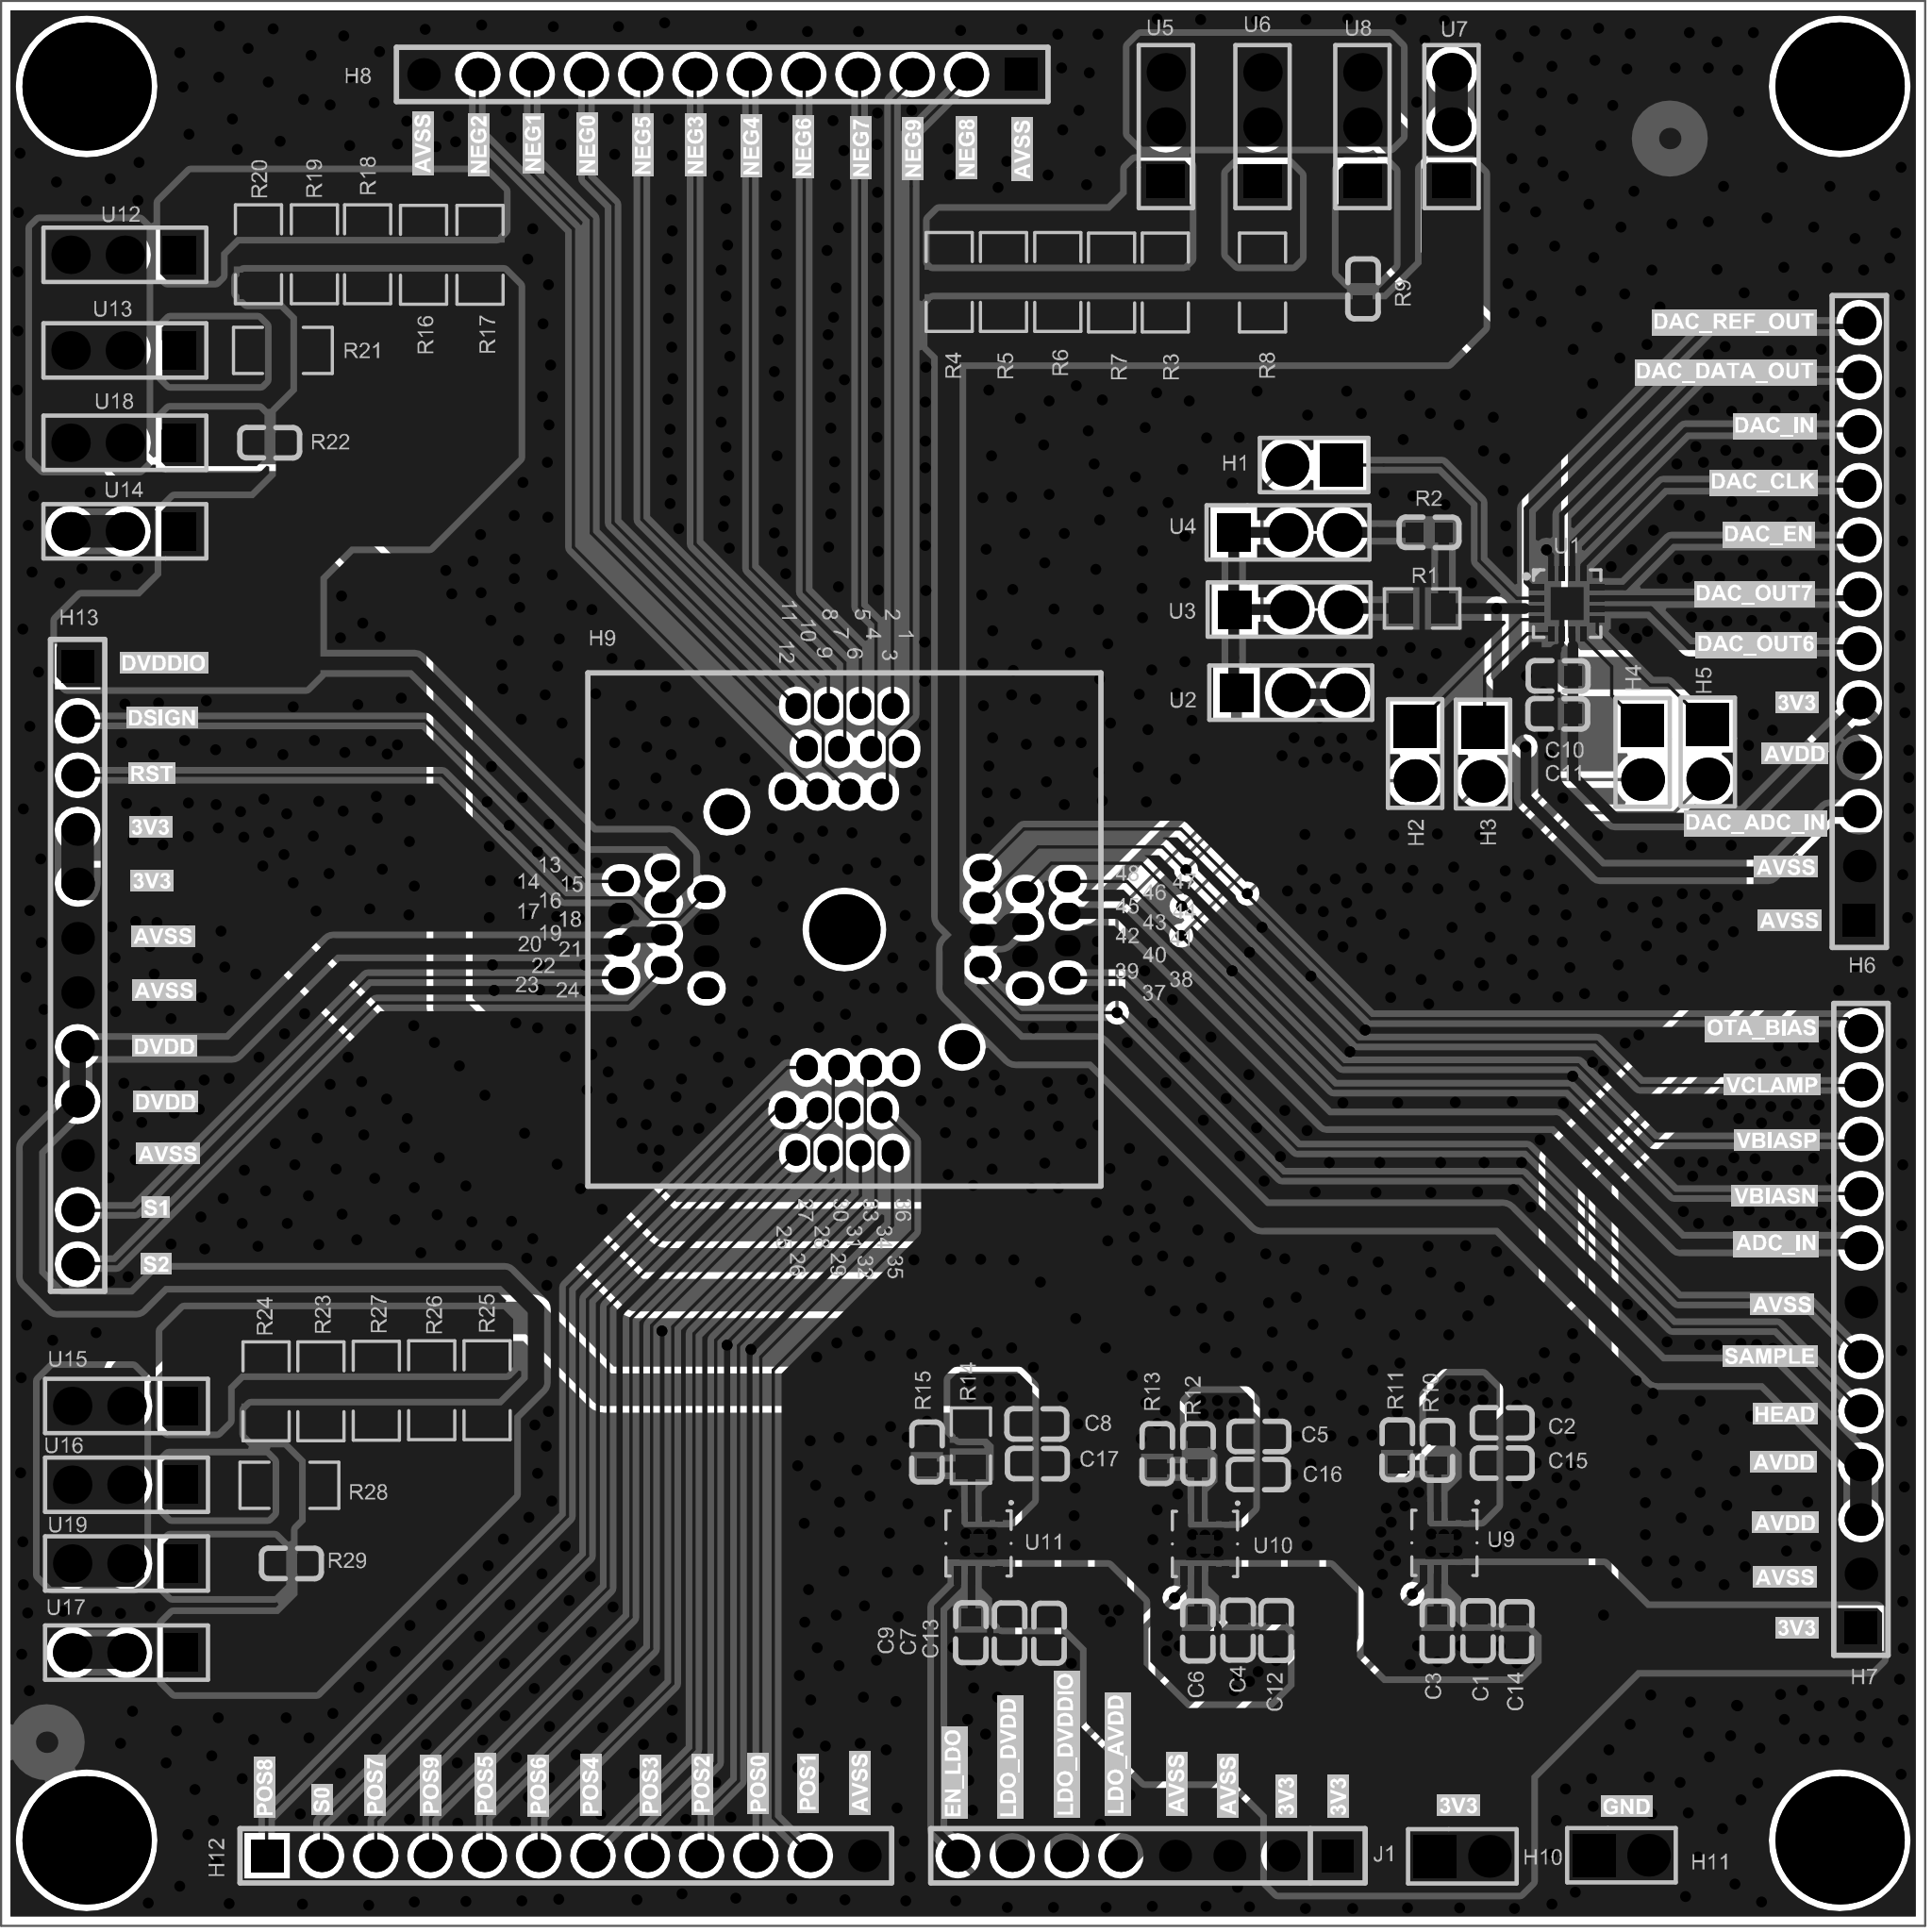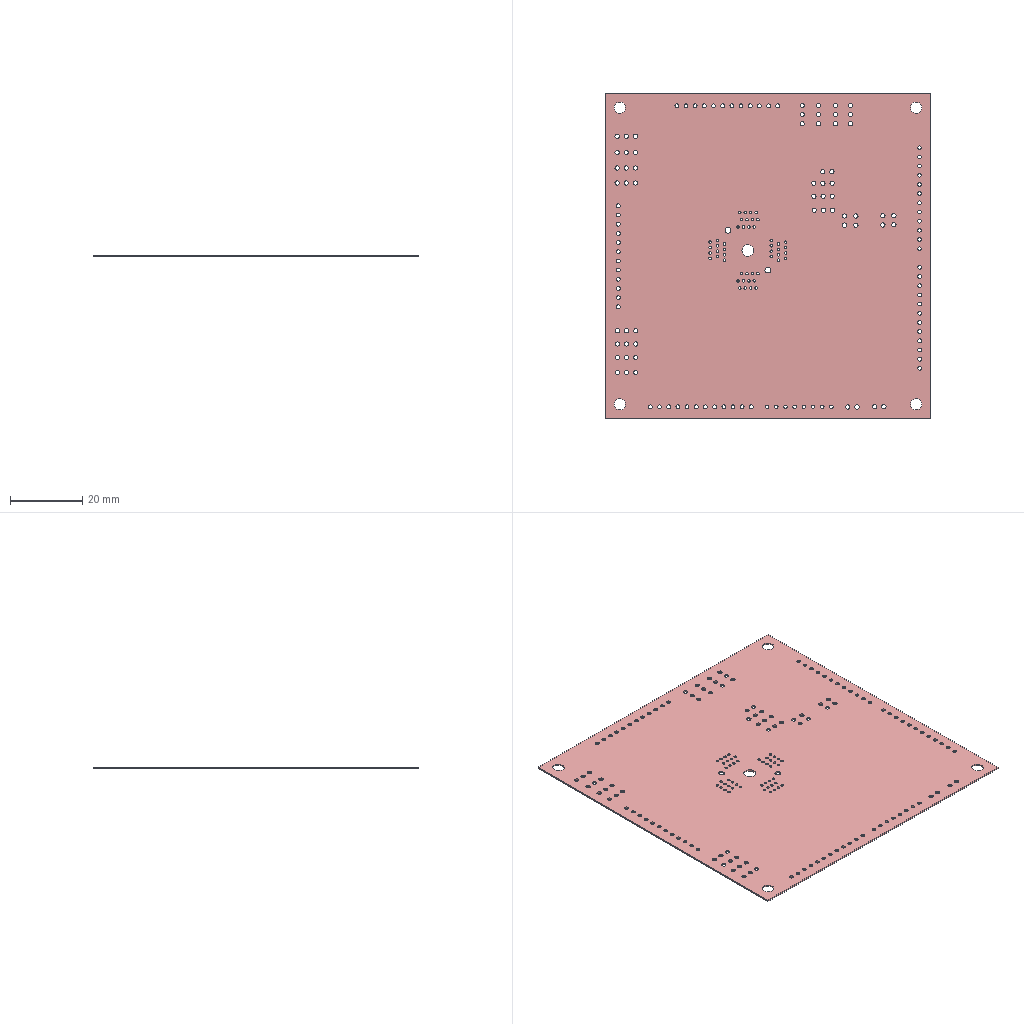Circuit board layout | Altium Designer | box 90 x 90 x 0.4 mm
Layer stack:
# Altium Designer layer stack of  (unit mm; dielectric type: 0 none, 1 core, 2 prepreg, 3 surface material)
index,name,kind,layer,copper_thickness_mm,dielectric_type,dielectric_thickness_mm,dielectric_material,dielectric_constant
0,Top Paste,other,,,,,,
1,Top Overlay,other,,,,,,
2,Top Solder,dielectric,,,3,0.0102,Solder Resist,3.5
3,Top Layer,copper,Top Layer,0.0356,,,,
4,Dielectric1,dielectric,,,0,0.32,FR-4,4.8
5,Bottom Layer,copper,Bottom Layer,0.0356,,,,
6,Bottom Solder,dielectric,,,3,0.0102,Solder Resist,3.5
7,Bottom Overlay,other,,,,,,
8,Bottom Paste,other,,,,,,
# drill layer pairs: low layer,high layer
drill_pair,Top Layer,Bottom Layer
Part placement:
Designator,Comment,Layer,Footprint,Center-X(mm),Center-Y(mm),Rotation
C17,4.7uF,TopLayer,C0603,48.463,21.615,180
C16,4.7uF,TopLayer,C0603,58.801,21.107,180
C15,4.7uF,TopLayer,C0603,70.206,21.641,180
C14,4.7uF,TopLayer,C0603,70.891,13.767,90
C13,4.7uF,TopLayer,C0603,49.022,13.691,90
C12,4.7uF,TopLayer,C0603,59.639,13.818,90
C11,100nF,TopLayer,C0603,72.822,56.667,360
C10,1uF,TopLayer,C0603,72.823,58.445,180
R28,10O,TopLayer,R1206,13.487,20.599,360
R27,10O,TopLayer,R1206,17.551,25.019,270
R26,10O,TopLayer,R1206,20.142,25.044,270
R25,10O,TopLayer,R1206,22.733,25.044,270
R24,10O,TopLayer,R1206,12.395,24.994,270
R23,10O,TopLayer,R1206,14.961,24.994,270
R21,10O,TopLayer,R1206,13.183,73.66,360
R20,10O,TopLayer,R1206,12.04,78.156,270
R19,10O,TopLayer,R1206,14.656,78.156,270
R18,10O,TopLayer,R1206,17.145,78.156,270
R17,10O,TopLayer,R1206,22.403,78.13,270
R16,10O,TopLayer,R1206,19.761,78.13,270
R8,10O,TopLayer,R1206,59.004,76.835,270
R7,10O,TopLayer,R1206,51.943,76.835,270
U19,2.54MM-1*3P 直针,TopLayer,HDR-TH_3P-P2.54-V-M-1,5.867,16.942,180
U18,2.54MM-1*3P 直针,TopLayer,HDR-TH_3P-P2.54-V-M-1,5.791,69.342,180
U17,2.54MM-1*3P 直针,TopLayer,HDR-TH_3P-P2.54-V-M-1,5.867,12.776,180
U16,2.54MM-1*3P 直针,TopLayer,HDR-TH_3P-P2.54-V-M-1,5.867,20.625,180
U15,2.54MM-1*3P 直针,TopLayer,HDR-TH_3P-P2.54-V-M-1,5.867,24.308,180
U14,2.54MM-1*3P 直针,TopLayer,HDR-TH_3P-P2.54-V-M-1,5.791,65.202,180
U13,2.54MM-1*3P 直针,TopLayer,HDR-TH_3P-P2.54-V-M-1,5.791,73.66,180
U12,2.54MM-1*3P 直针,TopLayer,HDR-TH_3P-P2.54-V-M-1,5.791,78.13,180
U11,TPS7A8001DRBR,TopLayer,VSON-8_L3.0-W3.0-P0.65-TL-EP,45.72,17.882,270
U10,TPS7A8001DRBR,TopLayer,VSON-8_L3.0-W3.0-P0.65-TL-EP,56.312,17.856,270
U9,TPS7A8001DRBR,TopLayer,VSON-8_L3.0-W3.0-P0.65-TL-EP,67.512,17.907,270
U8,2.54MM-1*3P 直针,TopLayer,HDR-TH_3P-P2.54-V-M-1,63.678,84.125,90
U7,2.54MM-1*3P 直针,TopLayer,HDR-TH_3P-P2.54-V-M-1,67.843,84.125,90
U6,2.54MM-1*3P 直针,TopLayer,HDR-TH_3P-P2.54-V-M-1,59.004,84.125,90
U5,2.54MM-1*3P 直针,TopLayer,HDR-TH_3P-P2.54-V-M-1,54.483,84.125,90
R29,118O,TopLayer,R0603,13.589,16.942,360
R22,118O,TopLayer,R0603,12.573,69.342,360
R15,10kO/1%,TopLayer,R0603,43.307,22.149,270
R14,1.25kO/1%,TopLayer,R0805,45.364,22.454,270
R13,10kO/1%,TopLayer,R0603,54.077,22.073,270
R12,12.6kO/1%,TopLayer,R0603,55.982,22.073,270
R11,10kO/1%,TopLayer,R0603,65.303,22.25,270
R10,12.6kO/1%,TopLayer,R0603,67.183,22.225,270
R9,118O,TopLayer,R0603,63.703,76.53,270
J1,Header2.54mm 1*8P,TopLayer,HDR-TH_8P-P2.54-V-M,53.645,3.277,180
H13,PZ254-1-12-Z-8.5,TopLayer,HDR-TH_12P-P2.54-V-M,3.581,44.907,270
H12,PZ254-1-12-Z-8.5,TopLayer,HDR-TH_12P-P2.54-V-M,26.416,3.277,360
H11,PZ254V-11-02P,TopLayer,HDR-TH_2P-P2.54-V-M,75.794,3.302,0
H10,PZ254V-11-02P,TopLayer,HDR-TH_2P-P2.54-V-M,68.351,3.251,0
H4,PZ254V-11-02P,TopLayer,HDR-TH_2P-P2.54-V-M,76.784,54.864,270
H3,PZ254V-11-02P,TopLayer,HDR-TH_2P-P2.54-V-M,69.317,54.788,270
H2,PZ254V-11-02P,TopLayer,HDR-TH_2P-P2.54-V-M,66.142,54.813,270
C1,1uF,TopLayer,C0603,69.088,13.792,270
C2,4.7uF,TopLayer,C0603,70.206,23.52,180
C3,10nF,TopLayer,C0603,67.183,13.792,90
C4,1uF,TopLayer,C0603,57.861,13.818,270
C5,4.7uF,TopLayer,C0603,58.826,22.885,180
C6,10nF,TopLayer,C0603,55.982,13.792,90
C7,1uF,TopLayer,C0603,47.168,13.691,270
C8,4.7uF,TopLayer,C0603,48.438,23.47,180
C9,10nF,TopLayer,C0603,45.364,13.716,90
H5,PZ254V-11-02P,TopLayer,HDR-TH_2P-P2.54-V-M,79.832,54.889,270
H6,PZ254-1-12-Z-8.5,TopLayer,HDR-TH_12P-P2.54-V-M,86.919,60.985,90
H7,PZ254-1-12-Z-8.5,TopLayer,HDR-TH_12P-P2.54-V-M,86.995,27.889,90
H8,PZ254-1-12-Z-8.5,TopLayer,HDR-TH_12P-P2.54-V-M,33.731,86.563,180
H9,TQPF-48-Z,TopLayer,TQPF-48-Z,39.446,46.584,270
R1,100kO,TopLayer,R0805,66.472,61.595,360
R2,10.5kO,TopLayer,R0603,66.802,65.151,360
R5,10O,TopLayer,R1206,46.888,76.86,270
R3,10O,TopLayer,R1206,54.458,76.835,270
R4,10O,TopLayer,R1206,44.348,76.86,270
R6,10O,TopLayer,R1206,49.428,76.86,270
U1,DAC60508ZRTER,TopLayer,WQFN-16_L3.0-W3.0-P0.50-BL-EP0.8,73.254,61.824,270
U2,2.54MM-1*3P 直针,TopLayer,HDR-TH_3P-P2.54-V-M-1,60.325,57.658,360
U3,2.54MM-1*3P 直针,TopLayer,HDR-TH_3P-P2.54-V-M-1,60.249,61.544,360
U4,2.54MM-1*3P 直针,TopLayer,HDR-TH_3P-P2.54-V-M-1,60.198,65.151,360
H1,PZ254V-11-02P,TopLayer,HDR-TH_2P-P2.54-V-M,61.417,68.301,180
Pad and via stacks:
# Altium Designer via and pad stacks of  (unit mm). Each distinct definition once, with the count of objects using it.
# via: kind,start_layer,end_layer,hole_mm,diameter_mm,mode(0 simple;1 top-mid-bottom;2 full stack),diameter_per_layer,count,example_net
# pad: kind,layer,hole_mm,hole_type(0 round;1 square;2 slot),plating,top_size,top_shape(1 round;2 rect;3 octagon;9 rounded rect),mid_size,bottom_size,mode,footprint,size_per_layer,count,example
pad,Top Layer,0,0,plated,0.34x0.8499,2,0.34x0.8499,0.34x0.8499,0,VSON-8_L3.0-W3.0-P0.65-TL-EP,,24,U9.8
pad,Top Layer,0,0,plated,0.8382x0.8382,2,0.8382x0.8382,0.8382x0.8382,0,VSON-8_L3.0-W3.0-P0.65-TL-EP,,3,U9.9
pad,Top Layer,0,0,plated,0.8x0.9,2,0.8x0.9,0.8x0.9,0,C0603,,34,C10.2
pad,Top Layer,0,0,plated,0.28x0.665,2,0.28x0.665,0.28x0.665,0,WQFN-16_L3.0-W3.0-P0.50-BL-EP0.8,,8,U1.1
pad,Top Layer,0,0,plated,0.665x0.28,2,0.665x0.28,0.665x0.28,0,WQFN-16_L3.0-W3.0-P0.50-BL-EP0.8,,8,U1.5
pad,Top Layer,0,0,plated,0.8x0.8,2,0.8x0.8,0.8x0.8,0,WQFN-16_L3.0-W3.0-P0.50-BL-EP0.8,,1,U1.17
pad,Top Layer,0,0,plated,1.133x1.377,2,1.133x1.377,1.133x1.377,0,R0805,,4,R14.2
pad,Top Layer,0,0,plated,0.8x0.9,2,0.8x0.9,0.8x0.9,0,R0603,,18,R29.2
pad,Top Layer,0,0,plated,1.208x1.701,2,1.208x1.701,1.208x1.701,0,R1206,,36,R28.2
pad,Top Layer,0,0,plated,1x1,1,1x1,1x1,0,,,2,MARK
pad,Multi-Layer,0.7,0,plated,1.2x1,1,1.2x1,1.2x1,0,TQPF-48-Z,,48,H9.24
pad,Multi-Layer,3.3,0,unplated,3.3x3.3,1,3.3x3.3,3.3x3.3,0,TQPF-48-Z,,1,H9.0
pad,Multi-Layer,1.6,0,unplated,1.6x1.6,1,1.6x1.6,1.6x1.6,0,TQPF-48-Z,,2,H9.0
pad,Multi-Layer,1.2,0,plated,2x2,2,2x2,2x2,0,HDR-TH_2P-P2.54-V-M,,7,H11.1
pad,Multi-Layer,1.2,0,plated,2x2,1,2x2,2x2,0,HDR-TH_2P-P2.54-V-M,,7,H11.2
pad,Multi-Layer,1.05,0,plated,1.524x1.524,2,1.524x1.524,1.524x1.524,0,HDR-TH_12P-P2.54-V-M,,5,H13.1
pad,Multi-Layer,1.05,0,plated,1.524x1.524,1,1.524x1.524,1.524x1.524,0,HDR-TH_12P-P2.54-V-M,,55,H13.2
pad,Multi-Layer,1,0,plated,1.5x1.5,2,1.5x1.5,1.5x1.5,0,HDR-TH_8P-P2.54-V-M,,1,J1.1
pad,Multi-Layer,1,0,plated,1.5x1.5,1,1.5x1.5,1.5x1.5,0,HDR-TH_8P-P2.54-V-M,,7,J1.2
pad,Multi-Layer,1.2,0,plated,1.8x1.8,1,1.8x1.8,1.8x1.8,0,HDR-TH_3P-P2.54-V-M-1,,30,U19.3
pad,Multi-Layer,1.2,0,plated,1.575x1.8,2,1.575x1.8,1.575x1.8,0,HDR-TH_3P-P2.54-V-M-1,,15,U19.1
pad,Multi-Layer,3.2,0,plated,6x6,1,6x6,6x6,0,,,4,0
via,Top Layer,Bottom Layer,0.3048,0.508,0,,1402,AVSS
Copper pours:
name,layer,net,type(0 solid;1 hatched;2 none)
Bottom Layer-No Net,Top Layer,AVSS,0
Bottom Layer-No Net,Top Layer,3.3V,0
Bottom Layer-No Net,Top Layer,LDO_AVDD,0
Bottom Layer-No Net,Top Layer,LDO_DVDDIO,0
Bottom Layer-No Net,Top Layer,LDO_DVDD,0
Bottom Layer-No Net,Top Layer,LDO_DVDDIO,0
Bottom Layer-No Net,Top Layer,DVDDIO,0
Bottom Layer-No Net,Top Layer,NetR22_1,0
Bottom Layer-No Net,Top Layer,NetR21_1,0
Bottom Layer-No Net,Top Layer,NetR16_1,0
Bottom Layer-No Net,Top Layer,LDO_DVDD,0
Bottom Layer-No Net,Top Layer,DVDD,0
Bottom Layer-No Net,Top Layer,NetR29_1,0
Bottom Layer-No Net,Top Layer,NetR28_1,0
Bottom Layer-No Net,Top Layer,NetR23_1,0
Bottom Layer-No Net,Top Layer,LDO_AVDD,0
Bottom Layer-No Net,Top Layer,NetR9_1,0
Bottom Layer-No Net,Top Layer,NetR8_1,0
Bottom Layer-No Net,Top Layer,AVDD,0
Bottom Layer-No Net,Top Layer,NetR3_1,0
Bottom Layer-No Net,Bottom Layer,AVSS,0
Bottom Layer-No Net,Bottom Layer,LDO_AVDD,0
Bottom Layer-No Net,Bottom Layer,LDO_DVDDIO,0
Bottom Layer-No Net,Bottom Layer,LDO_DVDD,0
Design rules, without the lines most boards share:
# Altium Designer design rules of  (exported by Altium Designer, unit mm)
# columns: name | kind | enabled | priority | scope1 | scope2 | descriptor | typed fields (field=value)
Clearance_2 | 0 | enabled | 1 | HASPAD('FREE-MARK') | All | Clearance Constraint (Gap=50mil) (HASPAD('FREE-MARK')),(All) | gap=1.27
Clearance_1 | 0 | enabled | 2 | INPOLYGON | All | Clearance Constraint (Gap=6mil) (INPOLYGON),(All) | gap=0.1524
Clearance | 0 | enabled | 3 | All | All | Clearance Constraint (Gap=6mil) (All),(All) | gap=0.1524
PlaneConnect | 6 | enabled | 1 | All | All | Power Plane Connect Rule(Direct Connect )(Expansion=20mil) (Conductor Width=10mil) (Air Gap=10mil) (Entries=4) (All) | relief_conductor_width=0.254 relief_entries=4 relief_expansion=0.508
PolygonConnect | 20 | enabled | 1 | All | All | Polygon Connect Rule(Direct Connect )(Conductor Width=10mil) (Relief Angle=90 Angle) (Entries=4) (Air Gap Width=10mil) (All),(All) | connect_style(0=relief,1=direct,2=none)=1 relief_conductor_width=0.254 relief_entries=4
Width | 2 | enabled | 1 | All | All | Width Constraint (Min=6mil) (Max=100mil) (Preferred=6mil) (All) |
RoutingVias | 11 | enabled | 1 | All | All | Routing Via (MinHoleWidth=12mil) (MaxHoleWidth=12mil) (PreferredHoleWidth=12mil) (MinWidth=20mil) (MaxWidth=20mil) (PreferedWidth=20mil) (All) | via_min_hole=0.3048 via_max_hole=0.3048 via_preferred_diameter=0.508 via_preferred_hole=0.3048
PasteMaskExpansion | 14 | enabled | 1 | All | All | Paste Mask Expansion (Expansion =0mil) (All) | expansion=0
SolderMaskExpansion | 13 | enabled | 1 | All | All | Solder Mask Expansion (Expansion =4mil) (All) | expansion=0.1016
HoleSize | 42 | enabled | 1 | All | All | Hole Size Constraint (Min=1mil) (Max=500mil) (All) |
DiffPairsRouting | 51 | enabled | 1 | All | All | Differential Pairs Uncoupled Length using the Gap Constraints (Min=10mil) (Max=10mil) (Prefered=10mil)  and Width Constraints (Min=15mil) (Max=15mil) (Prefered=15mil) (All) |
HoleToHoleClearance | 52 | enabled | 1 | All | All | Hole To Hole Clearance (Gap=0mil) (All),(All) | gap=0
MinimumSolderMaskSliver | 53 | enabled | 1 | All | All | Minimum Solder Mask Sliver (Gap=0mil) (All),(All) |
SilkscreenOverComponentPads | 54 | enabled | 1 | IsPad | All | Silk To Solder Mask (Clearance=0mil) (IsPad),(All) |
SilkToSilkClearance | 55 | enabled | 1 | All | All | Silk to Silk (Clearance=0mil) (All),(All) |
Classes set for this board:
# Altium Designer classes of  (member kind: 0 net, 1 component, 2 from-to, 3 pad, 4 layer, 5 differential pair, 6 design channel, 7 polygon, 8 structure, 9 xSignal)
# columns: class name | member kind | superclass | members
VCO_ADC_v2_2024-03-05 | 1 | no | C1; C2; C3; C4; C5; C6; C7; C8; C9; H1; H2; H3; H4; H5; H6; H7; H8; H9; R1; R2; R3; R4; R5; R6; U1; U2; U3; U4; H1; H2; H3; H4; H10; H11; H12; H13; J1; R9; R10; R11; R12; R13; R14; R15; R22; R29; U5; U6; U7; U8; U9; U10; U11; U12; U13; U14; U15; U16; U17; U18; U19; R7; R8; R16; R17; R18; R19; R20; R21; R23; R24; R25; R26; R27; R28; C10; C11; C12; C13; C14; C15; C16; C17;